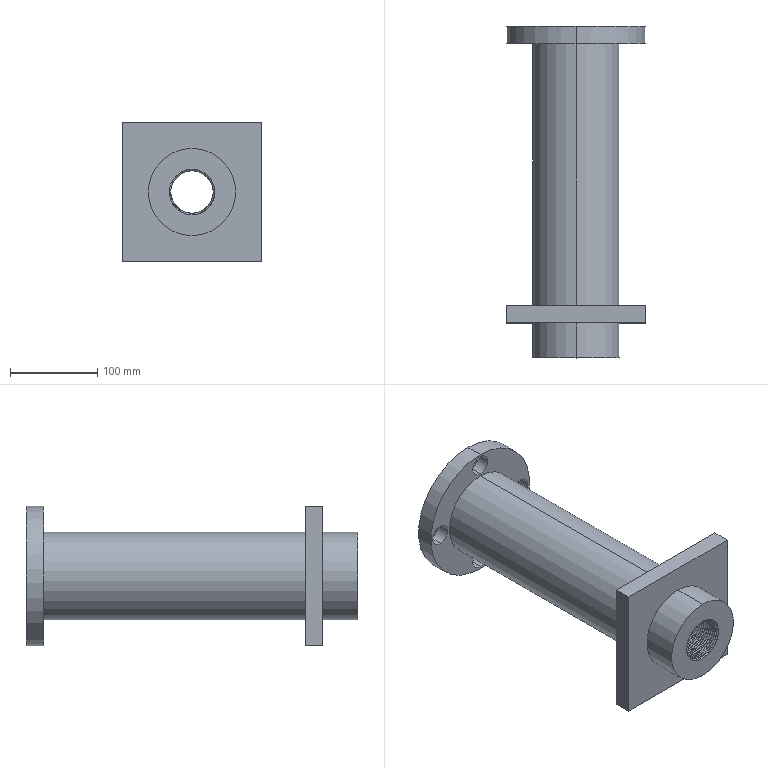Part | SolidWorks | features ICE 3, HoleWzd 2, Extrusion 1, SweepThread 1 | 1 solid | 293 faces | box 160 x 380 x 160 mm | volume 2803979 mm3 | cylinder 275 | plane 15 | spline 3 | commonest cylinder face diameters 52 x253 15.5 x8 24 x8 100 x4 160 x2